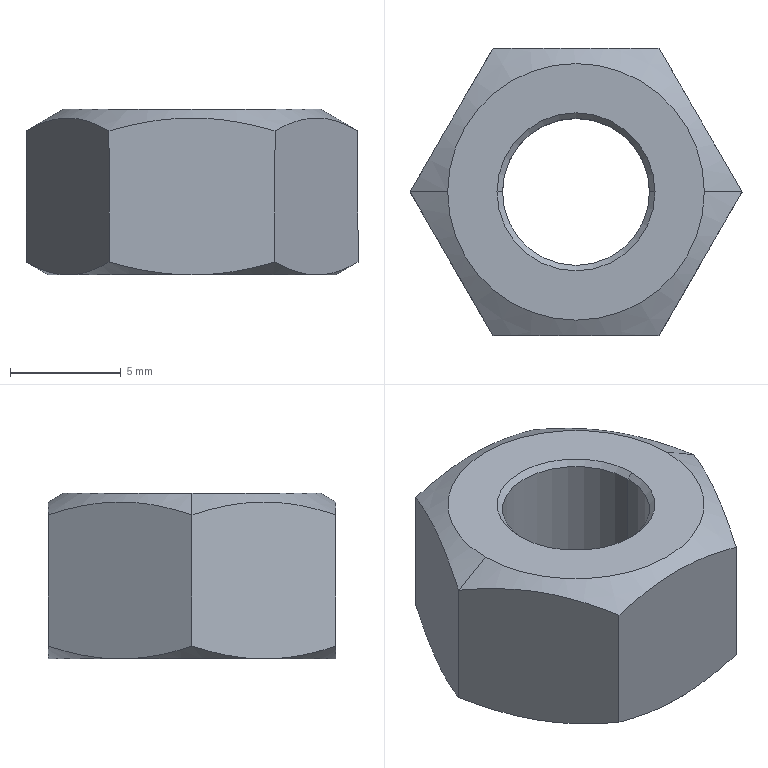Part | SolidWorks | features RevCut 4, Chamfer 2, Boss 1, Extrusion 1, LPattern 1 | 1 solid | 23 faces | box 15.011 x 13 x 7.5 mm | volume 813.544 mm3 | cone 13 | plane 8 | cylinder 2 | commonest cylinder face diameters 6.647 x2
STEP:
#1=CARTESIAN_POINT('',(-3.324,0.,-0.25));
#2=VERTEX_POINT('',#1);
#3=CARTESIAN_POINT('',(3.324,0.,-0.25));
#4=VERTEX_POINT('',#3);
#5=CARTESIAN_POINT('',(0.,0.,-0.25));
#6=DIRECTION('',(0.,0.,1.));
#7=DIRECTION('',(1.,0.,0.));
#8=AXIS2_PLACEMENT_3D('',#5,#6,#7);
#9=CIRCLE('',#8,3.324);
#10=EDGE_CURVE('',#2,#4,#9,.T.);
#11=ORIENTED_EDGE('',*,*,#10,.F.);
#12=CARTESIAN_POINT('',(-3.574,0.,0.));
#13=VERTEX_POINT('',#12);
#14=CARTESIAN_POINT('',(-3.324,0.,-0.25));
#15=DIRECTION('',(-0.7071,0.,0.7071));
#16=VECTOR('',#15,1000.);
#17=LINE('',#14,#16);
#18=EDGE_CURVE('',#2,#13,#17,.T.);
#19=ORIENTED_EDGE('',*,*,#18,.T.);
#20=CARTESIAN_POINT('',(3.574,0.,0.));
#21=VERTEX_POINT('',#20);
#22=CARTESIAN_POINT('',(0.,0.,0.));
#23=DIRECTION('',(0.,0.,-1.));
#24=DIRECTION('',(1.,0.,0.));
#25=AXIS2_PLACEMENT_3D('',#22,#23,#24);
#26=CIRCLE('',#25,3.574);
#27=EDGE_CURVE('',#21,#13,#26,.T.);
#28=ORIENTED_EDGE('',*,*,#27,.F.);
#29=CARTESIAN_POINT('',(3.324,0.,-0.25));
#30=DIRECTION('',(0.7071,0.,0.7071));
#31=VECTOR('',#30,1000.);
#32=LINE('',#29,#31);
#33=EDGE_CURVE('',#4,#21,#32,.T.);
#34=ORIENTED_EDGE('',*,*,#33,.F.);
#35=EDGE_LOOP('',(#11,#19,#28,#34));
#36=FACE_OUTER_BOUND('',#35,.T.);
#37=CARTESIAN_POINT('',(0.,0.,-0.25));
#38=DIRECTION('',(0.,0.,1.));
#39=DIRECTION('',(1.,0.,0.));
#40=AXIS2_PLACEMENT_3D('',#37,#38,#39);
#41=CONICAL_SURFACE('',#40,3.324,0.7854);
#42=ADVANCED_FACE('',(#36),#41,.F.);
#43=CARTESIAN_POINT('',(-5.8,0.,0.));
#44=VERTEX_POINT('',#43);
#45=CARTESIAN_POINT('',(5.8,0.,0.));
#46=VERTEX_POINT('',#45);
#47=CARTESIAN_POINT('',(0.,0.,0.));
#48=DIRECTION('',(0.,0.,-1.));
#49=DIRECTION('',(-1.,0.,0.));
#50=AXIS2_PLACEMENT_3D('',#47,#48,#49);
#51=CIRCLE('',#50,5.8);
#52=EDGE_CURVE('',#44,#46,#51,.T.);
#53=ORIENTED_EDGE('',*,*,#52,.T.);
#54=CARTESIAN_POINT('',(7.506,0.,-0.9847));
#55=VERTEX_POINT('',#54);
#56=CARTESIAN_POINT('',(7.506,0.,-0.9847));
#57=DIRECTION('',(0.866,0.,-0.5));
#58=VECTOR('',#57,1000.);
#59=LINE('',#56,#58);
#60=EDGE_CURVE('',#46,#55,#59,.T.);
#61=ORIENTED_EDGE('',*,*,#60,.T.);
#62=CARTESIAN_POINT('',(3.753,6.5,-0.9847));
#63=VERTEX_POINT('',#62);
#64=CARTESIAN_POINT('',(3.753,6.5,-0.9847));
#65=CARTESIAN_POINT('',(4.059,5.969,-0.8078));
#66=CARTESIAN_POINT('',(4.368,5.435,-0.662));
#67=CARTESIAN_POINT('',(4.991,4.355,-0.4601));
#68=CARTESIAN_POINT('',(5.307,3.809,-0.4046));
#69=CARTESIAN_POINT('',(5.785,2.98,-0.4039));
#70=CARTESIAN_POINT('',(5.945,2.702,-0.4175));
#71=CARTESIAN_POINT('',(6.262,2.153,-0.4704));
#72=CARTESIAN_POINT('',(6.42,1.88,-0.5097));
#73=CARTESIAN_POINT('',(6.889,1.067,-0.6614));
#74=CARTESIAN_POINT('',(7.199,0.5313,-0.8076));
#75=CARTESIAN_POINT('',(7.506,0.,-0.9847));
#76=B_SPLINE_CURVE_WITH_KNOTS('',3,(#64,#65,#66,#67,#68,#69,#70,#71,#72,#73,#74,#75),.UNSPECIFIED.,.F.,.F.,(4,2,2,2,2,4),(0.000000238,0.001895,0.00379,0.004738,0.005685,0.00758),.UNSPECIFIED.);
#77=EDGE_CURVE('',#63,#55,#76,.T.);
#78=ORIENTED_EDGE('',*,*,#77,.F.);
#79=CARTESIAN_POINT('',(-3.753,6.5,-0.9847));
#80=VERTEX_POINT('',#79);
#81=CARTESIAN_POINT('',(-3.753,6.5,-0.9847));
#82=CARTESIAN_POINT('',(-3.142,6.5,-0.8085));
#83=CARTESIAN_POINT('',(-2.517,6.5,-0.6607));
#84=CARTESIAN_POINT('',(-1.263,6.5,-0.4585));
#85=CARTESIAN_POINT('',(-0.6331,6.5,-0.4041));
#86=CARTESIAN_POINT('',(0.6352,6.5,-0.4042));
#87=CARTESIAN_POINT('',(1.278,6.5,-0.4602));
#88=CARTESIAN_POINT('',(2.532,6.5,-0.6637));
#89=CARTESIAN_POINT('',(3.146,6.5,-0.8096));
#90=CARTESIAN_POINT('',(3.753,6.5,-0.9847));
#91=B_SPLINE_CURVE_WITH_KNOTS('',3,(#81,#82,#83,#84,#85,#86,#87,#88,#89,#90),.UNSPECIFIED.,.F.,.F.,(4,2,2,2,4),(0.006633,0.008532,0.01043,0.01233,0.01423),.UNSPECIFIED.);
#92=EDGE_CURVE('',#80,#63,#91,.T.);
#93=ORIENTED_EDGE('',*,*,#92,.F.);
#94=CARTESIAN_POINT('',(-7.506,0.,-0.9847));
#95=VERTEX_POINT('',#94);
#96=CARTESIAN_POINT('',(-7.506,0.,-0.9847));
#97=CARTESIAN_POINT('',(-7.199,0.5307,-0.8078));
#98=CARTESIAN_POINT('',(-6.891,1.065,-0.662));
#99=CARTESIAN_POINT('',(-6.267,2.145,-0.4601));
#100=CARTESIAN_POINT('',(-5.952,2.691,-0.4046));
#101=CARTESIAN_POINT('',(-5.473,3.52,-0.4039));
#102=CARTESIAN_POINT('',(-5.313,3.798,-0.4175));
#103=CARTESIAN_POINT('',(-4.996,4.347,-0.4704));
#104=CARTESIAN_POINT('',(-4.838,4.62,-0.5097));
#105=CARTESIAN_POINT('',(-4.369,5.433,-0.6614));
#106=CARTESIAN_POINT('',(-4.06,5.969,-0.8076));
#107=CARTESIAN_POINT('',(-3.753,6.5,-0.9847));
#108=B_SPLINE_CURVE_WITH_KNOTS('',3,(#96,#97,#98,#99,#100,#101,#102,#103,#104,#105,#106,#107),.UNSPECIFIED.,.F.,.F.,(4,2,2,2,2,4),(0.000000238,0.001895,0.00379,0.004738,0.005685,0.00758),.UNSPECIFIED.);
#109=EDGE_CURVE('',#95,#80,#108,.T.);
#110=ORIENTED_EDGE('',*,*,#109,.F.);
#111=CARTESIAN_POINT('',(-7.506,0.,-0.9847));
#112=DIRECTION('',(-0.866,0.,-0.5));
#113=VECTOR('',#112,1000.);
#114=LINE('',#111,#113);
#115=EDGE_CURVE('',#44,#95,#114,.T.);
#116=ORIENTED_EDGE('',*,*,#115,.F.);
#117=EDGE_LOOP('',(#53,#61,#78,#93,#110,#116));
#118=FACE_OUTER_BOUND('',#117,.T.);
#119=CARTESIAN_POINT('',(0.,0.,-0.9847));
#120=DIRECTION('',(0.,0.,-1.));
#121=DIRECTION('',(-1.,0.,0.));
#122=AXIS2_PLACEMENT_3D('',#119,#120,#121);
#123=CONICAL_SURFACE('',#122,7.506,1.047);
#124=ADVANCED_FACE('',(#118),#123,.T.);
#125=CARTESIAN_POINT('',(-3.324,0.,-6.893));
#126=VERTEX_POINT('',#125);
#127=CARTESIAN_POINT('',(3.324,0.,-6.893));
#128=VERTEX_POINT('',#127);
#129=CARTESIAN_POINT('',(0.,0.,-6.893));
#130=DIRECTION('',(0.,0.,1.));
#131=DIRECTION('',(1.,0.,0.));
#132=AXIS2_PLACEMENT_3D('',#129,#130,#131);
#133=CIRCLE('',#132,3.324);
#134=EDGE_CURVE('',#126,#128,#133,.T.);
#135=ORIENTED_EDGE('',*,*,#134,.T.);
#136=CARTESIAN_POINT('',(4.375,0.,-7.5));
#137=VERTEX_POINT('',#136);
#138=CARTESIAN_POINT('',(3.324,0.,-6.893));
#139=DIRECTION('',(0.866,0.,-0.5));
#140=VECTOR('',#139,1000.);
#141=LINE('',#138,#140);
#142=EDGE_CURVE('',#128,#137,#141,.T.);
#143=ORIENTED_EDGE('',*,*,#142,.T.);
#144=CARTESIAN_POINT('',(-4.375,0.,-7.5));
#145=VERTEX_POINT('',#144);
#146=CARTESIAN_POINT('',(0.,0.,-7.5));
#147=DIRECTION('',(0.,0.,1.));
#148=DIRECTION('',(1.,0.,0.));
#149=AXIS2_PLACEMENT_3D('',#146,#147,#148);
#150=CIRCLE('',#149,4.375);
#151=EDGE_CURVE('',#145,#137,#150,.T.);
#152=ORIENTED_EDGE('',*,*,#151,.F.);
#153=CARTESIAN_POINT('',(-3.324,0.,-6.893));
#154=DIRECTION('',(-0.866,0.,-0.5));
#155=VECTOR('',#154,1000.);
#156=LINE('',#153,#155);
#157=EDGE_CURVE('',#126,#145,#156,.T.);
#158=ORIENTED_EDGE('',*,*,#157,.F.);
#159=EDGE_LOOP('',(#135,#143,#152,#158));
#160=FACE_OUTER_BOUND('',#159,.T.);
#161=CARTESIAN_POINT('',(0.,0.,-6.893));
#162=DIRECTION('',(0.,0.,-1.));
#163=DIRECTION('',(-1.,0.,0.));
#164=AXIS2_PLACEMENT_3D('',#161,#162,#163);
#165=CONICAL_SURFACE('',#164,3.324,1.047);
#166=ADVANCED_FACE('',(#160),#165,.F.);
#167=CARTESIAN_POINT('',(5.629,-3.25,-7.5));
#168=VERTEX_POINT('',#167);
#169=CARTESIAN_POINT('',(6.5,0.,-7.5));
#170=VERTEX_POINT('',#169);
#171=CARTESIAN_POINT('',(0.,0.,-7.5));
#172=DIRECTION('',(0.,0.,1.));
#173=DIRECTION('',(1.,0.,0.));
#174=AXIS2_PLACEMENT_3D('',#171,#172,#173);
#175=CIRCLE('',#174,6.5);
#176=EDGE_CURVE('',#168,#170,#175,.T.);
#177=ORIENTED_EDGE('',*,*,#176,.T.);
#178=CARTESIAN_POINT('',(7.506,0.,-6.919));
#179=VERTEX_POINT('',#178);
#180=CARTESIAN_POINT('',(7.506,0.,-6.919));
#181=DIRECTION('',(0.866,0.,0.5));
#182=VECTOR('',#181,1000.);
#183=LINE('',#180,#182);
#184=EDGE_CURVE('',#170,#179,#183,.T.);
#185=ORIENTED_EDGE('',*,*,#184,.T.);
#186=CARTESIAN_POINT('',(5.629,-3.25,-7.5));
#187=CARTESIAN_POINT('',(5.788,-2.974,-7.5));
#188=CARTESIAN_POINT('',(5.948,-2.697,-7.486));
#189=CARTESIAN_POINT('',(6.265,-2.149,-7.433));
#190=CARTESIAN_POINT('',(6.422,-1.877,-7.394));
#191=CARTESIAN_POINT('',(6.891,-1.065,-7.242));
#192=CARTESIAN_POINT('',(7.199,-0.5303,-7.096));
#193=CARTESIAN_POINT('',(7.506,0.,-6.919));
#194=B_SPLINE_CURVE_WITH_KNOTS('',3,(#186,#187,#188,#189,#190,#191,#192,#193),.UNSPECIFIED.,.F.,.F.,(4,2,2,4),(0.003797,0.004743,0.005689,0.00758),.UNSPECIFIED.);
#195=EDGE_CURVE('',#168,#179,#194,.T.);
#196=ORIENTED_EDGE('',*,*,#195,.F.);
#197=EDGE_LOOP('',(#177,#185,#196));
#198=FACE_OUTER_BOUND('',#197,.T.);
#199=CARTESIAN_POINT('',(0.,0.,-6.919));
#200=DIRECTION('',(0.,0.,1.));
#201=DIRECTION('',(1.,0.,0.));
#202=AXIS2_PLACEMENT_3D('',#199,#200,#201);
#203=CONICAL_SURFACE('',#202,7.506,1.047);
#204=ADVANCED_FACE('',(#198),#203,.T.);
#205=ORIENTED_EDGE('',*,*,#134,.F.);
#206=CARTESIAN_POINT('',(-3.324,0.,-7.5));
#207=DIRECTION('',(0.,0.,1.));
#208=VECTOR('',#207,1000.);
#209=LINE('',#206,#208);
#210=EDGE_CURVE('',#126,#2,#209,.T.);
#211=ORIENTED_EDGE('',*,*,#210,.T.);
#212=ORIENTED_EDGE('',*,*,#10,.T.);
#213=CARTESIAN_POINT('',(3.324,0.,-7.5));
#214=DIRECTION('',(0.,0.,1.));
#215=VECTOR('',#214,1000.);
#216=LINE('',#213,#215);
#217=EDGE_CURVE('',#128,#4,#216,.T.);
#218=ORIENTED_EDGE('',*,*,#217,.F.);
#219=EDGE_LOOP('',(#205,#211,#212,#218));
#220=FACE_OUTER_BOUND('',#219,.T.);
#221=CARTESIAN_POINT('',(0.,0.,-7.5));
#222=DIRECTION('',(0.,0.,1.));
#223=DIRECTION('',(1.,0.,0.));
#224=AXIS2_PLACEMENT_3D('',#221,#222,#223);
#225=CYLINDRICAL_SURFACE('',#224,3.324);
#226=ADVANCED_FACE('',(#220),#225,.F.);
#227=CARTESIAN_POINT('',(3.753,-6.5,-6.919));
#228=VERTEX_POINT('',#227);
#229=CARTESIAN_POINT('',(3.753,-6.5,-0.9847));
#230=VERTEX_POINT('',#229);
#231=CARTESIAN_POINT('',(3.753,-6.5,-7.5));
#232=DIRECTION('',(0.,0.,1.));
#233=VECTOR('',#232,1000.);
#234=LINE('',#231,#233);
#235=EDGE_CURVE('',#228,#230,#234,.T.);
#236=ORIENTED_EDGE('',*,*,#235,.T.);
#237=CARTESIAN_POINT('',(-3.753,-6.5,-0.9847));
#238=VERTEX_POINT('',#237);
#239=CARTESIAN_POINT('',(3.753,-6.5,-0.9847));
#240=CARTESIAN_POINT('',(3.146,-6.5,-0.8096));
#241=CARTESIAN_POINT('',(2.532,-6.5,-0.6637));
#242=CARTESIAN_POINT('',(1.278,-6.5,-0.4602));
#243=CARTESIAN_POINT('',(0.6352,-6.5,-0.4042));
#244=CARTESIAN_POINT('',(-0.6331,-6.5,-0.4041));
#245=CARTESIAN_POINT('',(-1.263,-6.5,-0.4585));
#246=CARTESIAN_POINT('',(-2.517,-6.5,-0.6607));
#247=CARTESIAN_POINT('',(-3.142,-6.5,-0.8085));
#248=CARTESIAN_POINT('',(-3.753,-6.5,-0.9847));
#249=B_SPLINE_CURVE_WITH_KNOTS('',3,(#239,#240,#241,#242,#243,#244,#245,#246,#247,#248),.UNSPECIFIED.,.F.,.F.,(4,2,2,2,4),(0.0167,0.0186,0.0205,0.0224,0.02431),.UNSPECIFIED.);
#250=EDGE_CURVE('',#230,#238,#249,.T.);
#251=ORIENTED_EDGE('',*,*,#250,.T.);
#252=CARTESIAN_POINT('',(-3.753,-6.5,-6.919));
#253=VERTEX_POINT('',#252);
#254=CARTESIAN_POINT('',(-3.753,-6.5,-7.5));
#255=DIRECTION('',(0.,0.,1.));
#256=VECTOR('',#255,1000.);
#257=LINE('',#254,#256);
#258=EDGE_CURVE('',#253,#238,#257,.T.);
#259=ORIENTED_EDGE('',*,*,#258,.F.);
#260=CARTESIAN_POINT('',(0.,-6.5,-7.5));
#261=VERTEX_POINT('',#260);
#262=CARTESIAN_POINT('',(-3.753,-6.5,-6.919));
#263=CARTESIAN_POINT('',(-3.142,-6.5,-7.096));
#264=CARTESIAN_POINT('',(-2.517,-6.5,-7.243));
#265=CARTESIAN_POINT('',(-1.264,-6.5,-7.445));
#266=CARTESIAN_POINT('',(-0.6342,-6.5,-7.5));
#267=CARTESIAN_POINT('',(0.,-6.5,-7.5));
#268=B_SPLINE_CURVE_WITH_KNOTS('',3,(#262,#263,#264,#265,#266,#267),.UNSPECIFIED.,.F.,.F.,(4,2,4),(0.006695,0.008594,0.01049),.UNSPECIFIED.);
#269=EDGE_CURVE('',#253,#261,#268,.T.);
#270=ORIENTED_EDGE('',*,*,#269,.T.);
#271=CARTESIAN_POINT('',(0.,-6.5,-7.5));
#272=CARTESIAN_POINT('',(0.6345,-6.5,-7.5));
#273=CARTESIAN_POINT('',(1.278,-6.5,-7.444));
#274=CARTESIAN_POINT('',(2.531,-6.5,-7.24));
#275=CARTESIAN_POINT('',(3.146,-6.5,-7.095));
#276=CARTESIAN_POINT('',(3.753,-6.5,-6.919));
#277=B_SPLINE_CURVE_WITH_KNOTS('',3,(#271,#272,#273,#274,#275,#276),.UNSPECIFIED.,.F.,.F.,(4,2,4),(0.01049,0.01239,0.01429),.UNSPECIFIED.);
#278=EDGE_CURVE('',#261,#228,#277,.T.);
#279=ORIENTED_EDGE('',*,*,#278,.T.);
#280=EDGE_LOOP('',(#236,#251,#259,#270,#279));
#281=FACE_OUTER_BOUND('',#280,.T.);
#282=CARTESIAN_POINT('',(-3.753,-6.5,-7.5));
#283=DIRECTION('',(0.,-1.,0.));
#284=DIRECTION('',(0.,0.,-1.));
#285=AXIS2_PLACEMENT_3D('',#282,#283,#284);
#286=PLANE('',#285);
#287=ADVANCED_FACE('',(#281),#286,.T.);
#288=ORIENTED_EDGE('',*,*,#258,.T.);
#289=CARTESIAN_POINT('',(-3.753,-6.5,-0.9847));
#290=CARTESIAN_POINT('',(-4.059,-5.969,-0.8078));
#291=CARTESIAN_POINT('',(-4.368,-5.435,-0.662));
#292=CARTESIAN_POINT('',(-4.991,-4.355,-0.4601));
#293=CARTESIAN_POINT('',(-5.307,-3.809,-0.4046));
#294=CARTESIAN_POINT('',(-5.785,-2.98,-0.4039));
#295=CARTESIAN_POINT('',(-5.945,-2.702,-0.4175));
#296=CARTESIAN_POINT('',(-6.262,-2.153,-0.4704));
#297=CARTESIAN_POINT('',(-6.42,-1.88,-0.5097));
#298=CARTESIAN_POINT('',(-6.889,-1.067,-0.6614));
#299=CARTESIAN_POINT('',(-7.199,-0.5313,-0.8076));
#300=CARTESIAN_POINT('',(-7.506,0.,-0.9847));
#301=B_SPLINE_CURVE_WITH_KNOTS('',3,(#289,#290,#291,#292,#293,#294,#295,#296,#297,#298,#299,#300),.UNSPECIFIED.,.F.,.F.,(4,2,2,2,2,4),(0.000000238,0.001895,0.00379,0.004738,0.005685,0.00758),.UNSPECIFIED.);
#302=EDGE_CURVE('',#238,#95,#301,.T.);
#303=ORIENTED_EDGE('',*,*,#302,.T.);
#304=CARTESIAN_POINT('',(-7.506,0.,-6.919));
#305=VERTEX_POINT('',#304);
#306=CARTESIAN_POINT('',(-7.506,0.,-7.5));
#307=DIRECTION('',(0.,0.,1.));
#308=VECTOR('',#307,1000.);
#309=LINE('',#306,#308);
#310=EDGE_CURVE('',#305,#95,#309,.T.);
#311=ORIENTED_EDGE('',*,*,#310,.F.);
#312=CARTESIAN_POINT('',(-5.629,-3.25,-7.5));
#313=VERTEX_POINT('',#312);
#314=CARTESIAN_POINT('',(-7.506,0.,-6.919));
#315=CARTESIAN_POINT('',(-7.199,-0.5317,-7.097));
#316=CARTESIAN_POINT('',(-6.889,-1.067,-7.243));
#317=CARTESIAN_POINT('',(-6.265,-2.149,-7.445));
#318=CARTESIAN_POINT('',(-5.949,-2.696,-7.5));
#319=CARTESIAN_POINT('',(-5.629,-3.25,-7.5));
#320=B_SPLINE_CURVE_WITH_KNOTS('',3,(#314,#315,#316,#317,#318,#319),.UNSPECIFIED.,.F.,.F.,(4,2,4),(0.000000238,0.001899,0.003797),.UNSPECIFIED.);
#321=EDGE_CURVE('',#305,#313,#320,.T.);
#322=ORIENTED_EDGE('',*,*,#321,.T.);
#323=CARTESIAN_POINT('',(-5.629,-3.25,-7.5));
#324=CARTESIAN_POINT('',(-5.47,-3.526,-7.5));
#325=CARTESIAN_POINT('',(-5.31,-3.803,-7.486));
#326=CARTESIAN_POINT('',(-4.994,-4.351,-7.433));
#327=CARTESIAN_POINT('',(-4.836,-4.623,-7.394));
#328=CARTESIAN_POINT('',(-4.368,-5.435,-7.242));
#329=CARTESIAN_POINT('',(-4.059,-5.97,-7.096));
#330=CARTESIAN_POINT('',(-3.753,-6.5,-6.919));
#331=B_SPLINE_CURVE_WITH_KNOTS('',3,(#323,#324,#325,#326,#327,#328,#329,#330),.UNSPECIFIED.,.F.,.F.,(4,2,2,4),(0.003797,0.004743,0.005689,0.00758),.UNSPECIFIED.);
#332=EDGE_CURVE('',#313,#253,#331,.T.);
#333=ORIENTED_EDGE('',*,*,#332,.T.);
#334=EDGE_LOOP('',(#288,#303,#311,#322,#333));
#335=FACE_OUTER_BOUND('',#334,.T.);
#336=CARTESIAN_POINT('',(-7.506,0.,-7.5));
#337=DIRECTION('',(-0.866,-0.5,0.));
#338=DIRECTION('',(0.5,-0.866,0.));
#339=AXIS2_PLACEMENT_3D('',#336,#337,#338);
#340=PLANE('',#339);
#341=ADVANCED_FACE('',(#335),#340,.T.);
#342=ORIENTED_EDGE('',*,*,#310,.T.);
#343=ORIENTED_EDGE('',*,*,#109,.T.);
#344=CARTESIAN_POINT('',(-3.753,6.5,-6.919));
#345=VERTEX_POINT('',#344);
#346=CARTESIAN_POINT('',(-3.753,6.5,-7.5));
#347=DIRECTION('',(0.,0.,1.));
#348=VECTOR('',#347,1000.);
#349=LINE('',#346,#348);
#350=EDGE_CURVE('',#345,#80,#349,.T.);
#351=ORIENTED_EDGE('',*,*,#350,.F.);
#352=CARTESIAN_POINT('',(-5.629,3.25,-7.5));
#353=VERTEX_POINT('',#352);
#354=CARTESIAN_POINT('',(-3.753,6.5,-6.919));
#355=CARTESIAN_POINT('',(-4.06,5.968,-7.097));
#356=CARTESIAN_POINT('',(-4.369,5.433,-7.243));
#357=CARTESIAN_POINT('',(-4.994,4.351,-7.445));
#358=CARTESIAN_POINT('',(-5.309,3.804,-7.5));
#359=CARTESIAN_POINT('',(-5.629,3.25,-7.5));
#360=B_SPLINE_CURVE_WITH_KNOTS('',3,(#354,#355,#356,#357,#358,#359),.UNSPECIFIED.,.F.,.F.,(4,2,4),(0.000000238,0.001899,0.003797),.UNSPECIFIED.);
#361=EDGE_CURVE('',#345,#353,#360,.T.);
#362=ORIENTED_EDGE('',*,*,#361,.T.);
#363=CARTESIAN_POINT('',(-5.629,3.25,-7.5));
#364=CARTESIAN_POINT('',(-5.788,2.974,-7.5));
#365=CARTESIAN_POINT('',(-5.948,2.697,-7.486));
#366=CARTESIAN_POINT('',(-6.265,2.149,-7.433));
#367=CARTESIAN_POINT('',(-6.422,1.877,-7.394));
#368=CARTESIAN_POINT('',(-6.891,1.065,-7.242));
#369=CARTESIAN_POINT('',(-7.199,0.5303,-7.096));
#370=CARTESIAN_POINT('',(-7.506,0.,-6.919));
#371=B_SPLINE_CURVE_WITH_KNOTS('',3,(#363,#364,#365,#366,#367,#368,#369,#370),.UNSPECIFIED.,.F.,.F.,(4,2,2,4),(0.003797,0.004743,0.005689,0.00758),.UNSPECIFIED.);
#372=EDGE_CURVE('',#353,#305,#371,.T.);
#373=ORIENTED_EDGE('',*,*,#372,.T.);
#374=EDGE_LOOP('',(#342,#343,#351,#362,#373));
#375=FACE_OUTER_BOUND('',#374,.T.);
#376=CARTESIAN_POINT('',(-3.753,6.5,-7.5));
#377=DIRECTION('',(-0.866,0.5,0.));
#378=DIRECTION('',(-0.5,-0.866,0.));
#379=AXIS2_PLACEMENT_3D('',#376,#377,#378);
#380=PLANE('',#379);
#381=ADVANCED_FACE('',(#375),#380,.T.);
#382=ORIENTED_EDGE('',*,*,#350,.T.);
#383=ORIENTED_EDGE('',*,*,#92,.T.);
#384=CARTESIAN_POINT('',(3.753,6.5,-6.919));
#385=VERTEX_POINT('',#384);
#386=CARTESIAN_POINT('',(3.753,6.5,-7.5));
#387=DIRECTION('',(0.,0.,1.));
#388=VECTOR('',#387,1000.);
#389=LINE('',#386,#388);
#390=EDGE_CURVE('',#385,#63,#389,.T.);
#391=ORIENTED_EDGE('',*,*,#390,.F.);
#392=CARTESIAN_POINT('',(0.,6.5,-7.5));
#393=VERTEX_POINT('',#392);
#394=CARTESIAN_POINT('',(3.753,6.5,-6.919));
#395=CARTESIAN_POINT('',(3.146,6.5,-7.095));
#396=CARTESIAN_POINT('',(2.531,6.5,-7.24));
#397=CARTESIAN_POINT('',(1.278,6.5,-7.444));
#398=CARTESIAN_POINT('',(0.6345,6.5,-7.5));
#399=CARTESIAN_POINT('',(0.,6.5,-7.5));
#400=B_SPLINE_CURVE_WITH_KNOTS('',3,(#394,#395,#396,#397,#398,#399),.UNSPECIFIED.,.F.,.F.,(4,2,4),(0.002751,0.004645,0.00654),.UNSPECIFIED.);
#401=EDGE_CURVE('',#385,#393,#400,.T.);
#402=ORIENTED_EDGE('',*,*,#401,.T.);
#403=CARTESIAN_POINT('',(0.,6.5,-7.5));
#404=CARTESIAN_POINT('',(-0.6342,6.5,-7.5));
#405=CARTESIAN_POINT('',(-1.264,6.5,-7.445));
#406=CARTESIAN_POINT('',(-2.517,6.5,-7.243));
#407=CARTESIAN_POINT('',(-3.142,6.5,-7.096));
#408=CARTESIAN_POINT('',(-3.753,6.5,-6.919));
#409=B_SPLINE_CURVE_WITH_KNOTS('',3,(#403,#404,#405,#406,#407,#408),.UNSPECIFIED.,.F.,.F.,(4,2,4),(0.00654,0.008433,0.01033),.UNSPECIFIED.);
#410=EDGE_CURVE('',#393,#345,#409,.T.);
#411=ORIENTED_EDGE('',*,*,#410,.T.);
#412=EDGE_LOOP('',(#382,#383,#391,#402,#411));
#413=FACE_OUTER_BOUND('',#412,.T.);
#414=CARTESIAN_POINT('',(3.753,6.5,-7.5));
#415=DIRECTION('',(0.,1.,0.));
#416=DIRECTION('',(0.,0.,1.));
#417=AXIS2_PLACEMENT_3D('',#414,#415,#416);
#418=PLANE('',#417);
#419=ADVANCED_FACE('',(#413),#418,.T.);
#420=ORIENTED_EDGE('',*,*,#390,.T.);
#421=ORIENTED_EDGE('',*,*,#77,.T.);
#422=CARTESIAN_POINT('',(7.506,0.,-7.5));
#423=DIRECTION('',(0.,0.,1.));
#424=VECTOR('',#423,1000.);
#425=LINE('',#422,#424);
#426=EDGE_CURVE('',#179,#55,#425,.T.);
#427=ORIENTED_EDGE('',*,*,#426,.F.);
#428=CARTESIAN_POINT('',(5.629,3.25,-7.5));
#429=VERTEX_POINT('',#428);
#430=CARTESIAN_POINT('',(7.506,0.,-6.919));
#431=CARTESIAN_POINT('',(7.199,0.5317,-7.097));
#432=CARTESIAN_POINT('',(6.889,1.067,-7.243));
#433=CARTESIAN_POINT('',(6.265,2.149,-7.445));
#434=CARTESIAN_POINT('',(5.949,2.696,-7.5));
#435=CARTESIAN_POINT('',(5.629,3.25,-7.5));
#436=B_SPLINE_CURVE_WITH_KNOTS('',3,(#430,#431,#432,#433,#434,#435),.UNSPECIFIED.,.F.,.F.,(4,2,4),(0.000000238,0.001899,0.003797),.UNSPECIFIED.);
#437=EDGE_CURVE('',#179,#429,#436,.T.);
#438=ORIENTED_EDGE('',*,*,#437,.T.);
#439=CARTESIAN_POINT('',(5.629,3.25,-7.5));
#440=CARTESIAN_POINT('',(5.47,3.526,-7.5));
#441=CARTESIAN_POINT('',(5.31,3.803,-7.486));
#442=CARTESIAN_POINT('',(4.994,4.351,-7.433));
#443=CARTESIAN_POINT('',(4.836,4.623,-7.394));
#444=CARTESIAN_POINT('',(4.368,5.435,-7.242));
#445=CARTESIAN_POINT('',(4.059,5.97,-7.096));
#446=CARTESIAN_POINT('',(3.753,6.5,-6.919));
#447=B_SPLINE_CURVE_WITH_KNOTS('',3,(#439,#440,#441,#442,#443,#444,#445,#446),.UNSPECIFIED.,.F.,.F.,(4,2,2,4),(0.003797,0.004743,0.005689,0.00758),.UNSPECIFIED.);
#448=EDGE_CURVE('',#429,#385,#447,.T.);
#449=ORIENTED_EDGE('',*,*,#448,.T.);
#450=EDGE_LOOP('',(#420,#421,#427,#438,#449));
#451=FACE_OUTER_BOUND('',#450,.T.);
#452=CARTESIAN_POINT('',(7.506,0.,-7.5));
#453=DIRECTION('',(0.866,0.5,0.));
#454=DIRECTION('',(-0.5,0.866,0.));
#455=AXIS2_PLACEMENT_3D('',#452,#453,#454);
#456=PLANE('',#455);
#457=ADVANCED_FACE('',(#451),#456,.T.);
#458=ORIENTED_EDGE('',*,*,#426,.T.);
#459=CARTESIAN_POINT('',(7.506,0.,-0.9847));
#460=CARTESIAN_POINT('',(7.199,-0.5307,-0.8078));
#461=CARTESIAN_POINT('',(6.891,-1.065,-0.662));
#462=CARTESIAN_POINT('',(6.267,-2.145,-0.4601));
#463=CARTESIAN_POINT('',(5.952,-2.691,-0.4046));
#464=CARTESIAN_POINT('',(5.473,-3.52,-0.4039));
#465=CARTESIAN_POINT('',(5.313,-3.798,-0.4175));
#466=CARTESIAN_POINT('',(4.996,-4.347,-0.4704));
#467=CARTESIAN_POINT('',(4.838,-4.62,-0.5097));
#468=CARTESIAN_POINT('',(4.369,-5.433,-0.6614));
#469=CARTESIAN_POINT('',(4.06,-5.969,-0.8076));
#470=CARTESIAN_POINT('',(3.753,-6.5,-0.9847));
#471=B_SPLINE_CURVE_WITH_KNOTS('',3,(#459,#460,#461,#462,#463,#464,#465,#466,#467,#468,#469,#470),.UNSPECIFIED.,.F.,.F.,(4,2,2,2,2,4),(0.000000238,0.001895,0.00379,0.004738,0.005685,0.00758),.UNSPECIFIED.);
#472=EDGE_CURVE('',#55,#230,#471,.T.);
#473=ORIENTED_EDGE('',*,*,#472,.T.);
#474=ORIENTED_EDGE('',*,*,#235,.F.);
#475=CARTESIAN_POINT('',(3.753,-6.5,-6.919));
#476=CARTESIAN_POINT('',(4.06,-5.968,-7.097));
#477=CARTESIAN_POINT('',(4.369,-5.433,-7.243));
#478=CARTESIAN_POINT('',(4.994,-4.351,-7.445));
#479=CARTESIAN_POINT('',(5.309,-3.804,-7.5));
#480=CARTESIAN_POINT('',(5.629,-3.25,-7.5));
#481=B_SPLINE_CURVE_WITH_KNOTS('',3,(#475,#476,#477,#478,#479,#480),.UNSPECIFIED.,.F.,.F.,(4,2,4),(0.000000238,0.001899,0.003797),.UNSPECIFIED.);
#482=EDGE_CURVE('',#228,#168,#481,.T.);
#483=ORIENTED_EDGE('',*,*,#482,.T.);
#484=ORIENTED_EDGE('',*,*,#195,.T.);
#485=EDGE_LOOP('',(#458,#473,#474,#483,#484));
#486=FACE_OUTER_BOUND('',#485,.T.);
#487=CARTESIAN_POINT('',(3.753,-6.5,-7.5));
#488=DIRECTION('',(0.866,-0.5,0.));
#489=DIRECTION('',(0.5,0.866,0.));
#490=AXIS2_PLACEMENT_3D('',#487,#488,#489);
#491=PLANE('',#490);
#492=ADVANCED_FACE('',(#486),#491,.T.);
#493=ORIENTED_EDGE('',*,*,#27,.T.);
#494=CARTESIAN_POINT('',(0.,0.,0.));
#495=DIRECTION('',(0.,0.,-1.));
#496=DIRECTION('',(1.,0.,0.));
#497=AXIS2_PLACEMENT_3D('',#494,#495,#496);
#498=CIRCLE('',#497,3.574);
#499=EDGE_CURVE('',#13,#21,#498,.T.);
#500=ORIENTED_EDGE('',*,*,#499,.T.);
#501=EDGE_LOOP('',(#493,#500));
#502=FACE_BOUND('',#501,.T.);
#503=ORIENTED_EDGE('',*,*,#52,.F.);
#504=CARTESIAN_POINT('',(0.,0.,0.));
#505=DIRECTION('',(0.,0.,-1.));
#506=DIRECTION('',(-1.,0.,0.));
#507=AXIS2_PLACEMENT_3D('',#504,#505,#506);
#508=CIRCLE('',#507,5.8);
#509=EDGE_CURVE('',#46,#44,#508,.T.);
#510=ORIENTED_EDGE('',*,*,#509,.F.);
#511=EDGE_LOOP('',(#503,#510));
#512=FACE_OUTER_BOUND('',#511,.T.);
#513=CARTESIAN_POINT('',(3.753,-6.5,0.));
#514=DIRECTION('',(0.,0.,1.));
#515=DIRECTION('',(1.,0.,0.));
#516=AXIS2_PLACEMENT_3D('',#513,#514,#515);
#517=PLANE('',#516);
#518=ADVANCED_FACE('',(#502,#512),#517,.T.);
#519=ORIENTED_EDGE('',*,*,#151,.T.);
#520=CARTESIAN_POINT('',(0.,0.,-7.5));
#521=DIRECTION('',(0.,0.,1.));
#522=DIRECTION('',(1.,0.,0.));
#523=AXIS2_PLACEMENT_3D('',#520,#521,#522);
#524=CIRCLE('',#523,4.375);
#525=EDGE_CURVE('',#137,#145,#524,.T.);
#526=ORIENTED_EDGE('',*,*,#525,.T.);
#527=EDGE_LOOP('',(#519,#526));
#528=FACE_BOUND('',#527,.T.);
#529=CARTESIAN_POINT('',(0.,0.,-7.5));
#530=DIRECTION('',(0.,0.,1.));
#531=DIRECTION('',(1.,0.,0.));
#532=AXIS2_PLACEMENT_3D('',#529,#530,#531);
#533=CIRCLE('',#532,6.5);
#534=EDGE_CURVE('',#429,#393,#533,.T.);
#535=ORIENTED_EDGE('',*,*,#534,.F.);
#536=CARTESIAN_POINT('',(0.,0.,-7.5));
#537=DIRECTION('',(0.,0.,1.));
#538=DIRECTION('',(1.,0.,0.));
#539=AXIS2_PLACEMENT_3D('',#536,#537,#538);
#540=CIRCLE('',#539,6.5);
#541=EDGE_CURVE('',#170,#429,#540,.T.);
#542=ORIENTED_EDGE('',*,*,#541,.F.);
#543=ORIENTED_EDGE('',*,*,#176,.F.);
#544=CARTESIAN_POINT('',(0.,0.,-7.5));
#545=DIRECTION('',(0.,0.,1.));
#546=DIRECTION('',(1.,0.,0.));
#547=AXIS2_PLACEMENT_3D('',#544,#545,#546);
#548=CIRCLE('',#547,6.5);
#549=EDGE_CURVE('',#261,#168,#548,.T.);
#550=ORIENTED_EDGE('',*,*,#549,.F.);
#551=CARTESIAN_POINT('',(0.,0.,-7.5));
#552=DIRECTION('',(0.,0.,1.));
#553=DIRECTION('',(1.,0.,0.));
#554=AXIS2_PLACEMENT_3D('',#551,#552,#553);
#555=CIRCLE('',#554,6.5);
#556=EDGE_CURVE('',#313,#261,#555,.T.);
#557=ORIENTED_EDGE('',*,*,#556,.F.);
#558=CARTESIAN_POINT('',(0.,0.,-7.5));
#559=DIRECTION('',(0.,0.,1.));
#560=DIRECTION('',(1.,0.,0.));
#561=AXIS2_PLACEMENT_3D('',#558,#559,#560);
#562=CIRCLE('',#561,6.5);
#563=EDGE_CURVE('',#353,#313,#562,.T.);
#564=ORIENTED_EDGE('',*,*,#563,.F.);
#565=CARTESIAN_POINT('',(0.,0.,-7.5));
#566=DIRECTION('',(0.,0.,1.));
#567=DIRECTION('',(1.,0.,0.));
#568=AXIS2_PLACEMENT_3D('',#565,#566,#567);
#569=CIRCLE('',#568,6.5);
#570=EDGE_CURVE('',#393,#353,#569,.T.);
#571=ORIENTED_EDGE('',*,*,#570,.F.);
#572=EDGE_LOOP('',(#535,#542,#543,#550,#557,#564,#571));
#573=FACE_OUTER_BOUND('',#572,.T.);
#574=CARTESIAN_POINT('',(3.753,-6.5,-7.5));
#575=DIRECTION('',(0.,0.,1.));
#576=DIRECTION('',(1.,0.,0.));
#577=AXIS2_PLACEMENT_3D('',#574,#575,#576);
#578=PLANE('',#577);
#579=ADVANCED_FACE('',(#528,#573),#578,.F.);
#580=ORIENTED_EDGE('',*,*,#210,.F.);
#581=CARTESIAN_POINT('',(0.,0.,-6.893));
#582=DIRECTION('',(0.,0.,1.));
#583=DIRECTION('',(1.,0.,0.));
#584=AXIS2_PLACEMENT_3D('',#581,#582,#583);
#585=CIRCLE('',#584,3.324);
#586=EDGE_CURVE('',#128,#126,#585,.T.);
#587=ORIENTED_EDGE('',*,*,#586,.F.);
#588=ORIENTED_EDGE('',*,*,#217,.T.);
#589=CARTESIAN_POINT('',(0.,0.,-0.25));
#590=DIRECTION('',(0.,0.,1.));
#591=DIRECTION('',(1.,0.,0.));
#592=AXIS2_PLACEMENT_3D('',#589,#590,#591);
#593=CIRCLE('',#592,3.324);
#594=EDGE_CURVE('',#4,#2,#593,.T.);
#595=ORIENTED_EDGE('',*,*,#594,.T.);
#596=EDGE_LOOP('',(#580,#587,#588,#595));
#597=FACE_OUTER_BOUND('',#596,.T.);
#598=CARTESIAN_POINT('',(0.,0.,-7.5));
#599=DIRECTION('',(0.,0.,1.));
#600=DIRECTION('',(1.,0.,0.));
#601=AXIS2_PLACEMENT_3D('',#598,#599,#600);
#602=CYLINDRICAL_SURFACE('',#601,3.324);
#603=ADVANCED_FACE('',(#597),#602,.F.);
#604=ORIENTED_EDGE('',*,*,#184,.F.);
#605=ORIENTED_EDGE('',*,*,#541,.T.);
#606=ORIENTED_EDGE('',*,*,#437,.F.);
#607=EDGE_LOOP('',(#604,#605,#606));
#608=FACE_OUTER_BOUND('',#607,.T.);
#609=CARTESIAN_POINT('',(0.,0.,-6.919));
#610=DIRECTION('',(0.,0.,1.));
#611=DIRECTION('',(1.,0.,0.));
#612=AXIS2_PLACEMENT_3D('',#609,#610,#611);
#613=CONICAL_SURFACE('',#612,7.506,1.047);
#614=ADVANCED_FACE('',(#608),#613,.T.);
#615=ORIENTED_EDGE('',*,*,#549,.T.);
#616=ORIENTED_EDGE('',*,*,#482,.F.);
#617=ORIENTED_EDGE('',*,*,#278,.F.);
#618=EDGE_LOOP('',(#615,#616,#617));
#619=FACE_OUTER_BOUND('',#618,.T.);
#620=CARTESIAN_POINT('',(0.,0.,-6.919));
#621=DIRECTION('',(0.,0.,1.));
#622=DIRECTION('',(1.,0.,0.));
#623=AXIS2_PLACEMENT_3D('',#620,#621,#622);
#624=CONICAL_SURFACE('',#623,7.506,1.047);
#625=ADVANCED_FACE('',(#619),#624,.T.);
#626=ORIENTED_EDGE('',*,*,#556,.T.);
#627=ORIENTED_EDGE('',*,*,#269,.F.);
#628=ORIENTED_EDGE('',*,*,#332,.F.);
#629=EDGE_LOOP('',(#626,#627,#628));
#630=FACE_OUTER_BOUND('',#629,.T.);
#631=CARTESIAN_POINT('',(0.,0.,-6.919));
#632=DIRECTION('',(0.,0.,1.));
#633=DIRECTION('',(1.,0.,0.));
#634=AXIS2_PLACEMENT_3D('',#631,#632,#633);
#635=CONICAL_SURFACE('',#634,7.506,1.047);
#636=ADVANCED_FACE('',(#630),#635,.T.);
#637=ORIENTED_EDGE('',*,*,#563,.T.);
#638=ORIENTED_EDGE('',*,*,#321,.F.);
#639=ORIENTED_EDGE('',*,*,#372,.F.);
#640=EDGE_LOOP('',(#637,#638,#639));
#641=FACE_OUTER_BOUND('',#640,.T.);
#642=CARTESIAN_POINT('',(0.,0.,-6.919));
#643=DIRECTION('',(0.,0.,1.));
#644=DIRECTION('',(1.,0.,0.));
#645=AXIS2_PLACEMENT_3D('',#642,#643,#644);
#646=CONICAL_SURFACE('',#645,7.506,1.047);
#647=ADVANCED_FACE('',(#641),#646,.T.);
#648=ORIENTED_EDGE('',*,*,#410,.F.);
#649=ORIENTED_EDGE('',*,*,#570,.T.);
#650=ORIENTED_EDGE('',*,*,#361,.F.);
#651=EDGE_LOOP('',(#648,#649,#650));
#652=FACE_OUTER_BOUND('',#651,.T.);
#653=CARTESIAN_POINT('',(0.,0.,-6.919));
#654=DIRECTION('',(0.,0.,1.));
#655=DIRECTION('',(1.,0.,0.));
#656=AXIS2_PLACEMENT_3D('',#653,#654,#655);
#657=CONICAL_SURFACE('',#656,7.506,1.047);
#658=ADVANCED_FACE('',(#652),#657,.T.);
#659=ORIENTED_EDGE('',*,*,#448,.F.);
#660=ORIENTED_EDGE('',*,*,#534,.T.);
#661=ORIENTED_EDGE('',*,*,#401,.F.);
#662=EDGE_LOOP('',(#659,#660,#661));
#663=FACE_OUTER_BOUND('',#662,.T.);
#664=CARTESIAN_POINT('',(0.,0.,-6.919));
#665=DIRECTION('',(0.,0.,1.));
#666=DIRECTION('',(1.,0.,0.));
#667=AXIS2_PLACEMENT_3D('',#664,#665,#666);
#668=CONICAL_SURFACE('',#667,7.506,1.047);
#669=ADVANCED_FACE('',(#663),#668,.T.);
#670=ORIENTED_EDGE('',*,*,#142,.F.);
#671=ORIENTED_EDGE('',*,*,#586,.T.);
#672=ORIENTED_EDGE('',*,*,#157,.T.);
#673=ORIENTED_EDGE('',*,*,#525,.F.);
#674=EDGE_LOOP('',(#670,#671,#672,#673));
#675=FACE_OUTER_BOUND('',#674,.T.);
#676=CARTESIAN_POINT('',(0.,0.,-6.893));
#677=DIRECTION('',(0.,0.,-1.));
#678=DIRECTION('',(-1.,0.,0.));
#679=AXIS2_PLACEMENT_3D('',#676,#677,#678);
#680=CONICAL_SURFACE('',#679,3.324,1.047);
#681=ADVANCED_FACE('',(#675),#680,.F.);
#682=ORIENTED_EDGE('',*,*,#60,.F.);
#683=ORIENTED_EDGE('',*,*,#509,.T.);
#684=ORIENTED_EDGE('',*,*,#115,.T.);
#685=ORIENTED_EDGE('',*,*,#302,.F.);
#686=ORIENTED_EDGE('',*,*,#250,.F.);
#687=ORIENTED_EDGE('',*,*,#472,.F.);
#688=EDGE_LOOP('',(#682,#683,#684,#685,#686,#687));
#689=FACE_OUTER_BOUND('',#688,.T.);
#690=CARTESIAN_POINT('',(0.,0.,-0.9847));
#691=DIRECTION('',(0.,0.,-1.));
#692=DIRECTION('',(-1.,0.,0.));
#693=AXIS2_PLACEMENT_3D('',#690,#691,#692);
#694=CONICAL_SURFACE('',#693,7.506,1.047);
#695=ADVANCED_FACE('',(#689),#694,.T.);
#696=ORIENTED_EDGE('',*,*,#18,.F.);
#697=ORIENTED_EDGE('',*,*,#594,.F.);
#698=ORIENTED_EDGE('',*,*,#33,.T.);
#699=ORIENTED_EDGE('',*,*,#499,.F.);
#700=EDGE_LOOP('',(#696,#697,#698,#699));
#701=FACE_OUTER_BOUND('',#700,.T.);
#702=CARTESIAN_POINT('',(0.,0.,-0.25));
#703=DIRECTION('',(0.,0.,1.));
#704=DIRECTION('',(1.,0.,0.));
#705=AXIS2_PLACEMENT_3D('',#702,#703,#704);
#706=CONICAL_SURFACE('',#705,3.324,0.7854);
#707=ADVANCED_FACE('',(#701),#706,.F.);
#708=CLOSED_SHELL('',(#42,#124,#166,#204,#226,#287,#341,#381,#419,#457,#492,#518,#579,#603,#614,#625,#636,#647,#658,#669,#681,#695,#707));
#709=MANIFOLD_SOLID_BREP('',#708);
#710=CARTESIAN_POINT('',(0.,0.,0.));
#711=DIRECTION('',(0.,0.,1.));
#712=DIRECTION('',(1.,0.,0.));
#713=AXIS2_PLACEMENT_3D('',#710,#711,#712);
#714=(LENGTH_UNIT()NAMED_UNIT(*)SI_UNIT(.MILLI.,.METRE.));
#715=UNCERTAINTY_MEASURE_WITH_UNIT(LENGTH_MEASURE(0.00001),#714,'','');
#716=(NAMED_UNIT(*)PLANE_ANGLE_UNIT()SI_UNIT($,.RADIAN.));
#717=(NAMED_UNIT(*)SI_UNIT($,.STERADIAN.)SOLID_ANGLE_UNIT());
#718=(GEOMETRIC_REPRESENTATION_CONTEXT(3)GLOBAL_UNCERTAINTY_ASSIGNED_CONTEXT((#715))GLOBAL_UNIT_ASSIGNED_CONTEXT((#714,#716,#717))REPRESENTATION_CONTEXT('',''));
#719=ADVANCED_BREP_SHAPE_REPRESENTATION('',(#709,#713),#718);